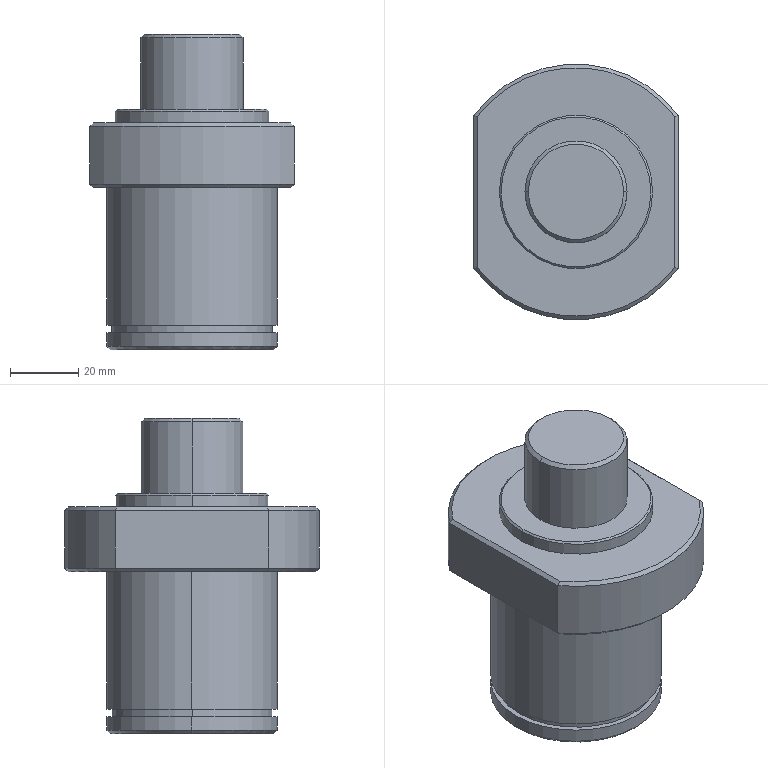Part | SolidWorks | features ICE 7, Chamfer 3, Extrusion 1 | 1 solid | 35 faces | box 60 x 75 x 92.5 mm | volume 189510 mm3 | plane 13 | cylinder 12 | cone 10 | commonest cylinder face diameters 50 x4 30 x2 45 x2 47 x2 75 x2
STEP:
#1=CARTESIAN_POINT('',(25.,0.,-79.5));
#2=VERTEX_POINT('',#1);
#3=CARTESIAN_POINT('',(-25.,0.,-79.5));
#4=VERTEX_POINT('',#3);
#5=CARTESIAN_POINT('',(0.,0.,-79.5));
#6=DIRECTION('',(0.,0.,1.));
#7=DIRECTION('',(-1.,0.,0.));
#8=AXIS2_PLACEMENT_3D('',#5,#6,#7);
#9=CIRCLE('',#8,25.);
#10=EDGE_CURVE('',#2,#4,#9,.T.);
#11=ORIENTED_EDGE('',*,*,#10,.T.);
#12=CARTESIAN_POINT('',(-25.,0.,-75.5));
#13=VERTEX_POINT('',#12);
#14=CARTESIAN_POINT('',(-25.,0.,-80.5));
#15=DIRECTION('',(0.,0.,1.));
#16=VECTOR('',#15,1000.);
#17=LINE('',#14,#16);
#18=EDGE_CURVE('',#4,#13,#17,.T.);
#19=ORIENTED_EDGE('',*,*,#18,.T.);
#20=CARTESIAN_POINT('',(25.,0.,-75.5));
#21=VERTEX_POINT('',#20);
#22=CARTESIAN_POINT('',(0.,0.,-75.5));
#23=DIRECTION('',(0.,0.,-1.));
#24=DIRECTION('',(-1.,0.,0.));
#25=AXIS2_PLACEMENT_3D('',#22,#23,#24);
#26=CIRCLE('',#25,25.);
#27=EDGE_CURVE('',#13,#21,#26,.T.);
#28=ORIENTED_EDGE('',*,*,#27,.T.);
#29=CARTESIAN_POINT('',(25.,0.,-80.5));
#30=DIRECTION('',(0.,0.,1.));
#31=VECTOR('',#30,1000.);
#32=LINE('',#29,#31);
#33=EDGE_CURVE('',#2,#21,#32,.T.);
#34=ORIENTED_EDGE('',*,*,#33,.F.);
#35=EDGE_LOOP('',(#11,#19,#28,#34));
#36=FACE_OUTER_BOUND('',#35,.T.);
#37=CARTESIAN_POINT('',(0.,0.,-80.5));
#38=DIRECTION('',(0.,0.,1.));
#39=DIRECTION('',(1.,0.,0.));
#40=AXIS2_PLACEMENT_3D('',#37,#38,#39);
#41=CYLINDRICAL_SURFACE('',#40,25.);
#42=ADVANCED_FACE('',(#36),#41,.T.);
#43=CARTESIAN_POINT('',(-24.,0.,-80.5));
#44=VERTEX_POINT('',#43);
#45=CARTESIAN_POINT('',(24.,0.,-80.5));
#46=VERTEX_POINT('',#45);
#47=CARTESIAN_POINT('',(0.,0.,-80.5));
#48=DIRECTION('',(0.,0.,-1.));
#49=DIRECTION('',(-1.,0.,0.));
#50=AXIS2_PLACEMENT_3D('',#47,#48,#49);
#51=CIRCLE('',#50,24.);
#52=EDGE_CURVE('',#44,#46,#51,.T.);
#53=ORIENTED_EDGE('',*,*,#52,.F.);
#54=CARTESIAN_POINT('',(-24.,0.,-80.5));
#55=DIRECTION('',(-0.7071,0.,0.7071));
#56=VECTOR('',#55,1000.);
#57=LINE('',#54,#56);
#58=EDGE_CURVE('',#44,#4,#57,.T.);
#59=ORIENTED_EDGE('',*,*,#58,.T.);
#60=ORIENTED_EDGE('',*,*,#10,.F.);
#61=CARTESIAN_POINT('',(24.,0.,-80.5));
#62=DIRECTION('',(0.7071,0.,0.7071));
#63=VECTOR('',#62,1000.);
#64=LINE('',#61,#63);
#65=EDGE_CURVE('',#46,#2,#64,.T.);
#66=ORIENTED_EDGE('',*,*,#65,.F.);
#67=EDGE_LOOP('',(#53,#59,#60,#66));
#68=FACE_OUTER_BOUND('',#67,.T.);
#69=CARTESIAN_POINT('',(0.,0.,-80.5));
#70=DIRECTION('',(0.,0.,1.));
#71=DIRECTION('',(1.,0.,0.));
#72=AXIS2_PLACEMENT_3D('',#69,#70,#71);
#73=CONICAL_SURFACE('',#72,24.,0.7854);
#74=ADVANCED_FACE('',(#68),#73,.T.);
#75=CARTESIAN_POINT('',(-23.5,0.,-73.3));
#76=VERTEX_POINT('',#75);
#77=CARTESIAN_POINT('',(23.5,0.,-73.3));
#78=VERTEX_POINT('',#77);
#79=CARTESIAN_POINT('',(0.,0.,-73.3));
#80=DIRECTION('',(0.,0.,-1.));
#81=DIRECTION('',(-1.,0.,0.));
#82=AXIS2_PLACEMENT_3D('',#79,#80,#81);
#83=CIRCLE('',#82,23.5);
#84=EDGE_CURVE('',#76,#78,#83,.T.);
#85=ORIENTED_EDGE('',*,*,#84,.T.);
#86=CARTESIAN_POINT('',(23.5,0.,-75.5));
#87=VERTEX_POINT('',#86);
#88=CARTESIAN_POINT('',(23.5,0.,-73.3));
#89=DIRECTION('',(0.,0.,-1.));
#90=VECTOR('',#89,1000.);
#91=LINE('',#88,#90);
#92=EDGE_CURVE('',#78,#87,#91,.T.);
#93=ORIENTED_EDGE('',*,*,#92,.T.);
#94=CARTESIAN_POINT('',(-23.5,0.,-75.5));
#95=VERTEX_POINT('',#94);
#96=CARTESIAN_POINT('',(0.,0.,-75.5));
#97=DIRECTION('',(0.,0.,-1.));
#98=DIRECTION('',(-1.,0.,0.));
#99=AXIS2_PLACEMENT_3D('',#96,#97,#98);
#100=CIRCLE('',#99,23.5);
#101=EDGE_CURVE('',#95,#87,#100,.T.);
#102=ORIENTED_EDGE('',*,*,#101,.F.);
#103=CARTESIAN_POINT('',(-23.5,0.,-73.3));
#104=DIRECTION('',(0.,0.,-1.));
#105=VECTOR('',#104,1000.);
#106=LINE('',#103,#105);
#107=EDGE_CURVE('',#76,#95,#106,.T.);
#108=ORIENTED_EDGE('',*,*,#107,.F.);
#109=EDGE_LOOP('',(#85,#93,#102,#108));
#110=FACE_OUTER_BOUND('',#109,.T.);
#111=CARTESIAN_POINT('',(0.,0.,-73.3));
#112=DIRECTION('',(0.,0.,-1.));
#113=DIRECTION('',(-1.,0.,0.));
#114=AXIS2_PLACEMENT_3D('',#111,#112,#113);
#115=CYLINDRICAL_SURFACE('',#114,23.5);
#116=ADVANCED_FACE('',(#110),#115,.T.);
#117=CARTESIAN_POINT('',(22.,0.,-10.));
#118=VERTEX_POINT('',#117);
#119=CARTESIAN_POINT('',(-22.,0.,-10.));
#120=VERTEX_POINT('',#119);
#121=CARTESIAN_POINT('',(0.,0.,-10.));
#122=DIRECTION('',(0.,0.,1.));
#123=DIRECTION('',(1.,0.,0.));
#124=AXIS2_PLACEMENT_3D('',#121,#122,#123);
#125=CIRCLE('',#124,22.);
#126=EDGE_CURVE('',#118,#120,#125,.T.);
#127=ORIENTED_EDGE('',*,*,#126,.F.);
#128=CARTESIAN_POINT('',(22.5,0.,-10.5));
#129=VERTEX_POINT('',#128);
#130=CARTESIAN_POINT('',(22.,0.,-10.));
#131=DIRECTION('',(0.7071,0.,-0.7071));
#132=VECTOR('',#131,1000.);
#133=LINE('',#130,#132);
#134=EDGE_CURVE('',#118,#129,#133,.T.);
#135=ORIENTED_EDGE('',*,*,#134,.T.);
#136=CARTESIAN_POINT('',(-22.5,0.,-10.5));
#137=VERTEX_POINT('',#136);
#138=CARTESIAN_POINT('',(0.,0.,-10.5));
#139=DIRECTION('',(0.,0.,-1.));
#140=DIRECTION('',(1.,0.,0.));
#141=AXIS2_PLACEMENT_3D('',#138,#139,#140);
#142=CIRCLE('',#141,22.5);
#143=EDGE_CURVE('',#137,#129,#142,.T.);
#144=ORIENTED_EDGE('',*,*,#143,.F.);
#145=CARTESIAN_POINT('',(-22.,0.,-10.));
#146=DIRECTION('',(-0.7071,0.,-0.7071));
#147=VECTOR('',#146,1000.);
#148=LINE('',#145,#147);
#149=EDGE_CURVE('',#120,#137,#148,.T.);
#150=ORIENTED_EDGE('',*,*,#149,.F.);
#151=EDGE_LOOP('',(#127,#135,#144,#150));
#152=FACE_OUTER_BOUND('',#151,.T.);
#153=CARTESIAN_POINT('',(0.,0.,-10.));
#154=DIRECTION('',(0.,0.,-1.));
#155=DIRECTION('',(-1.,0.,0.));
#156=AXIS2_PLACEMENT_3D('',#153,#154,#155);
#157=CONICAL_SURFACE('',#156,22.,0.7854);
#158=ADVANCED_FACE('',(#152),#157,.T.);
#159=CARTESIAN_POINT('',(14.,0.,12.));
#160=VERTEX_POINT('',#159);
#161=CARTESIAN_POINT('',(-14.,0.,12.));
#162=VERTEX_POINT('',#161);
#163=CARTESIAN_POINT('',(0.,0.,12.));
#164=DIRECTION('',(0.,0.,1.));
#165=DIRECTION('',(1.,0.,0.));
#166=AXIS2_PLACEMENT_3D('',#163,#164,#165);
#167=CIRCLE('',#166,14.);
#168=EDGE_CURVE('',#160,#162,#167,.T.);
#169=ORIENTED_EDGE('',*,*,#168,.F.);
#170=CARTESIAN_POINT('',(15.,0.,11.));
#171=VERTEX_POINT('',#170);
#172=CARTESIAN_POINT('',(14.,0.,12.));
#173=DIRECTION('',(0.7071,0.,-0.7071));
#174=VECTOR('',#173,1000.);
#175=LINE('',#172,#174);
#176=EDGE_CURVE('',#160,#171,#175,.T.);
#177=ORIENTED_EDGE('',*,*,#176,.T.);
#178=CARTESIAN_POINT('',(-15.,0.,11.));
#179=VERTEX_POINT('',#178);
#180=CARTESIAN_POINT('',(0.,0.,11.));
#181=DIRECTION('',(0.,0.,-1.));
#182=DIRECTION('',(1.,0.,0.));
#183=AXIS2_PLACEMENT_3D('',#180,#181,#182);
#184=CIRCLE('',#183,15.);
#185=EDGE_CURVE('',#179,#171,#184,.T.);
#186=ORIENTED_EDGE('',*,*,#185,.F.);
#187=CARTESIAN_POINT('',(-14.,0.,12.));
#188=DIRECTION('',(-0.7071,0.,-0.7071));
#189=VECTOR('',#188,1000.);
#190=LINE('',#187,#189);
#191=EDGE_CURVE('',#162,#179,#190,.T.);
#192=ORIENTED_EDGE('',*,*,#191,.F.);
#193=EDGE_LOOP('',(#169,#177,#186,#192));
#194=FACE_OUTER_BOUND('',#193,.T.);
#195=CARTESIAN_POINT('',(0.,0.,12.));
#196=DIRECTION('',(0.,0.,-1.));
#197=DIRECTION('',(-1.,0.,0.));
#198=AXIS2_PLACEMENT_3D('',#195,#196,#197);
#199=CONICAL_SURFACE('',#198,14.,0.7854);
#200=ADVANCED_FACE('',(#194),#199,.T.);
#201=ORIENTED_EDGE('',*,*,#185,.T.);
#202=CARTESIAN_POINT('',(15.,0.,-10.));
#203=VERTEX_POINT('',#202);
#204=CARTESIAN_POINT('',(15.,0.,12.));
#205=DIRECTION('',(0.,0.,-1.));
#206=VECTOR('',#205,1000.);
#207=LINE('',#204,#206);
#208=EDGE_CURVE('',#171,#203,#207,.T.);
#209=ORIENTED_EDGE('',*,*,#208,.T.);
#210=CARTESIAN_POINT('',(-15.,0.,-10.));
#211=VERTEX_POINT('',#210);
#212=CARTESIAN_POINT('',(0.,0.,-10.));
#213=DIRECTION('',(0.,0.,1.));
#214=DIRECTION('',(1.,0.,0.));
#215=AXIS2_PLACEMENT_3D('',#212,#213,#214);
#216=CIRCLE('',#215,15.);
#217=EDGE_CURVE('',#203,#211,#216,.T.);
#218=ORIENTED_EDGE('',*,*,#217,.T.);
#219=CARTESIAN_POINT('',(-15.,0.,12.));
#220=DIRECTION('',(0.,0.,-1.));
#221=VECTOR('',#220,1000.);
#222=LINE('',#219,#221);
#223=EDGE_CURVE('',#179,#211,#222,.T.);
#224=ORIENTED_EDGE('',*,*,#223,.F.);
#225=EDGE_LOOP('',(#201,#209,#218,#224));
#226=FACE_OUTER_BOUND('',#225,.T.);
#227=CARTESIAN_POINT('',(0.,0.,12.));
#228=DIRECTION('',(0.,0.,-1.));
#229=DIRECTION('',(-1.,0.,0.));
#230=AXIS2_PLACEMENT_3D('',#227,#228,#229);
#231=CYLINDRICAL_SURFACE('',#230,15.);
#232=ADVANCED_FACE('',(#226),#231,.T.);
#233=ORIENTED_EDGE('',*,*,#143,.T.);
#234=CARTESIAN_POINT('',(22.5,0.,-14.));
#235=VERTEX_POINT('',#234);
#236=CARTESIAN_POINT('',(22.5,0.,-10.));
#237=DIRECTION('',(0.,0.,-1.));
#238=VECTOR('',#237,1000.);
#239=LINE('',#236,#238);
#240=EDGE_CURVE('',#129,#235,#239,.T.);
#241=ORIENTED_EDGE('',*,*,#240,.T.);
#242=CARTESIAN_POINT('',(-22.5,0.,-14.));
#243=VERTEX_POINT('',#242);
#244=CARTESIAN_POINT('',(0.,0.,-14.));
#245=DIRECTION('',(0.,0.,1.));
#246=DIRECTION('',(1.,0.,0.));
#247=AXIS2_PLACEMENT_3D('',#244,#245,#246);
#248=CIRCLE('',#247,22.5);
#249=EDGE_CURVE('',#235,#243,#248,.T.);
#250=ORIENTED_EDGE('',*,*,#249,.T.);
#251=CARTESIAN_POINT('',(-22.5,0.,-10.));
#252=DIRECTION('',(0.,0.,-1.));
#253=VECTOR('',#252,1000.);
#254=LINE('',#251,#253);
#255=EDGE_CURVE('',#137,#243,#254,.T.);
#256=ORIENTED_EDGE('',*,*,#255,.F.);
#257=EDGE_LOOP('',(#233,#241,#250,#256));
#258=FACE_OUTER_BOUND('',#257,.T.);
#259=CARTESIAN_POINT('',(0.,0.,-10.));
#260=DIRECTION('',(0.,0.,-1.));
#261=DIRECTION('',(-1.,0.,0.));
#262=AXIS2_PLACEMENT_3D('',#259,#260,#261);
#263=CYLINDRICAL_SURFACE('',#262,22.5);
#264=ADVANCED_FACE('',(#258),#263,.T.);
#265=CARTESIAN_POINT('',(-25.,0.,-73.3));
#266=VERTEX_POINT('',#265);
#267=CARTESIAN_POINT('',(25.,0.,-73.3));
#268=VERTEX_POINT('',#267);
#269=CARTESIAN_POINT('',(0.,0.,-73.3));
#270=DIRECTION('',(0.,0.,-1.));
#271=DIRECTION('',(-1.,0.,0.));
#272=AXIS2_PLACEMENT_3D('',#269,#270,#271);
#273=CIRCLE('',#272,25.);
#274=EDGE_CURVE('',#266,#268,#273,.T.);
#275=ORIENTED_EDGE('',*,*,#274,.F.);
#276=CARTESIAN_POINT('',(-25.,0.,-33.));
#277=VERTEX_POINT('',#276);
#278=CARTESIAN_POINT('',(-25.,0.,-80.5));
#279=DIRECTION('',(0.,0.,1.));
#280=VECTOR('',#279,1000.);
#281=LINE('',#278,#280);
#282=EDGE_CURVE('',#266,#277,#281,.T.);
#283=ORIENTED_EDGE('',*,*,#282,.T.);
#284=CARTESIAN_POINT('',(25.,0.,-33.));
#285=VERTEX_POINT('',#284);
#286=CARTESIAN_POINT('',(0.,0.,-33.));
#287=DIRECTION('',(0.,0.,1.));
#288=DIRECTION('',(1.,0.,0.));
#289=AXIS2_PLACEMENT_3D('',#286,#287,#288);
#290=CIRCLE('',#289,25.);
#291=EDGE_CURVE('',#285,#277,#290,.T.);
#292=ORIENTED_EDGE('',*,*,#291,.F.);
#293=CARTESIAN_POINT('',(25.,0.,-80.5));
#294=DIRECTION('',(0.,0.,1.));
#295=VECTOR('',#294,1000.);
#296=LINE('',#293,#295);
#297=EDGE_CURVE('',#268,#285,#296,.T.);
#298=ORIENTED_EDGE('',*,*,#297,.F.);
#299=EDGE_LOOP('',(#275,#283,#292,#298));
#300=FACE_OUTER_BOUND('',#299,.T.);
#301=CARTESIAN_POINT('',(0.,0.,-80.5));
#302=DIRECTION('',(0.,0.,1.));
#303=DIRECTION('',(1.,0.,0.));
#304=AXIS2_PLACEMENT_3D('',#301,#302,#303);
#305=CYLINDRICAL_SURFACE('',#304,25.);
#306=ADVANCED_FACE('',(#300),#305,.T.);
#307=ORIENTED_EDGE('',*,*,#282,.F.);
#308=CARTESIAN_POINT('',(0.,0.,-73.3));
#309=DIRECTION('',(0.,0.,-1.));
#310=DIRECTION('',(-1.,0.,0.));
#311=AXIS2_PLACEMENT_3D('',#308,#309,#310);
#312=CIRCLE('',#311,25.);
#313=EDGE_CURVE('',#268,#266,#312,.T.);
#314=ORIENTED_EDGE('',*,*,#313,.F.);
#315=ORIENTED_EDGE('',*,*,#297,.T.);
#316=CARTESIAN_POINT('',(0.,0.,-33.));
#317=DIRECTION('',(0.,0.,1.));
#318=DIRECTION('',(1.,0.,0.));
#319=AXIS2_PLACEMENT_3D('',#316,#317,#318);
#320=CIRCLE('',#319,25.);
#321=EDGE_CURVE('',#277,#285,#320,.T.);
#322=ORIENTED_EDGE('',*,*,#321,.F.);
#323=EDGE_LOOP('',(#307,#314,#315,#322));
#324=FACE_OUTER_BOUND('',#323,.T.);
#325=CARTESIAN_POINT('',(0.,0.,-80.5));
#326=DIRECTION('',(0.,0.,1.));
#327=DIRECTION('',(1.,0.,0.));
#328=AXIS2_PLACEMENT_3D('',#325,#326,#327);
#329=CYLINDRICAL_SURFACE('',#328,25.);
#330=ADVANCED_FACE('',(#324),#329,.T.);
#331=ORIENTED_EDGE('',*,*,#240,.F.);
#332=CARTESIAN_POINT('',(0.,0.,-10.5));
#333=DIRECTION('',(0.,0.,-1.));
#334=DIRECTION('',(1.,0.,0.));
#335=AXIS2_PLACEMENT_3D('',#332,#333,#334);
#336=CIRCLE('',#335,22.5);
#337=EDGE_CURVE('',#129,#137,#336,.T.);
#338=ORIENTED_EDGE('',*,*,#337,.T.);
#339=ORIENTED_EDGE('',*,*,#255,.T.);
#340=CARTESIAN_POINT('',(0.,0.,-14.));
#341=DIRECTION('',(0.,0.,1.));
#342=DIRECTION('',(1.,0.,0.));
#343=AXIS2_PLACEMENT_3D('',#340,#341,#342);
#344=CIRCLE('',#343,22.5);
#345=EDGE_CURVE('',#243,#235,#344,.T.);
#346=ORIENTED_EDGE('',*,*,#345,.T.);
#347=EDGE_LOOP('',(#331,#338,#339,#346));
#348=FACE_OUTER_BOUND('',#347,.T.);
#349=CARTESIAN_POINT('',(0.,0.,-10.));
#350=DIRECTION('',(0.,0.,-1.));
#351=DIRECTION('',(-1.,0.,0.));
#352=AXIS2_PLACEMENT_3D('',#349,#350,#351);
#353=CYLINDRICAL_SURFACE('',#352,22.5);
#354=ADVANCED_FACE('',(#348),#353,.T.);
#355=CARTESIAN_POINT('',(0.,0.,-10.));
#356=DIRECTION('',(0.,0.,1.));
#357=DIRECTION('',(1.,0.,0.));
#358=AXIS2_PLACEMENT_3D('',#355,#356,#357);
#359=CIRCLE('',#358,22.);
#360=EDGE_CURVE('',#120,#118,#359,.T.);
#361=ORIENTED_EDGE('',*,*,#360,.T.);
#362=ORIENTED_EDGE('',*,*,#126,.T.);
#363=EDGE_LOOP('',(#361,#362));
#364=FACE_OUTER_BOUND('',#363,.T.);
#365=CARTESIAN_POINT('',(0.,0.,-10.));
#366=DIRECTION('',(0.,0.,1.));
#367=DIRECTION('',(1.,0.,0.));
#368=AXIS2_PLACEMENT_3D('',#365,#366,#367);
#369=CIRCLE('',#368,15.);
#370=EDGE_CURVE('',#211,#203,#369,.T.);
#371=ORIENTED_EDGE('',*,*,#370,.F.);
#372=ORIENTED_EDGE('',*,*,#217,.F.);
#373=EDGE_LOOP('',(#371,#372));
#374=FACE_BOUND('',#373,.T.);
#375=CARTESIAN_POINT('',(0.,0.,-10.));
#376=DIRECTION('',(0.,0.,1.));
#377=DIRECTION('',(1.,0.,0.));
#378=AXIS2_PLACEMENT_3D('',#375,#376,#377);
#379=PLANE('',#378);
#380=ADVANCED_FACE('',(#364,#374),#379,.T.);
#381=CARTESIAN_POINT('',(0.,0.,12.));
#382=DIRECTION('',(0.,0.,1.));
#383=DIRECTION('',(1.,0.,0.));
#384=AXIS2_PLACEMENT_3D('',#381,#382,#383);
#385=CIRCLE('',#384,14.);
#386=EDGE_CURVE('',#162,#160,#385,.T.);
#387=ORIENTED_EDGE('',*,*,#386,.T.);
#388=ORIENTED_EDGE('',*,*,#168,.T.);
#389=EDGE_LOOP('',(#387,#388));
#390=FACE_OUTER_BOUND('',#389,.T.);
#391=CARTESIAN_POINT('',(0.,0.,12.));
#392=DIRECTION('',(0.,0.,1.));
#393=DIRECTION('',(1.,0.,0.));
#394=AXIS2_PLACEMENT_3D('',#391,#392,#393);
#395=PLANE('',#394);
#396=ADVANCED_FACE('',(#390),#395,.T.);
#397=ORIENTED_EDGE('',*,*,#208,.F.);
#398=CARTESIAN_POINT('',(0.,0.,11.));
#399=DIRECTION('',(0.,0.,-1.));
#400=DIRECTION('',(1.,0.,0.));
#401=AXIS2_PLACEMENT_3D('',#398,#399,#400);
#402=CIRCLE('',#401,15.);
#403=EDGE_CURVE('',#171,#179,#402,.T.);
#404=ORIENTED_EDGE('',*,*,#403,.T.);
#405=ORIENTED_EDGE('',*,*,#223,.T.);
#406=ORIENTED_EDGE('',*,*,#370,.T.);
#407=EDGE_LOOP('',(#397,#404,#405,#406));
#408=FACE_OUTER_BOUND('',#407,.T.);
#409=CARTESIAN_POINT('',(0.,0.,12.));
#410=DIRECTION('',(0.,0.,-1.));
#411=DIRECTION('',(-1.,0.,0.));
#412=AXIS2_PLACEMENT_3D('',#409,#410,#411);
#413=CYLINDRICAL_SURFACE('',#412,15.);
#414=ADVANCED_FACE('',(#408),#413,.T.);
#415=ORIENTED_EDGE('',*,*,#176,.F.);
#416=ORIENTED_EDGE('',*,*,#386,.F.);
#417=ORIENTED_EDGE('',*,*,#191,.T.);
#418=ORIENTED_EDGE('',*,*,#403,.F.);
#419=EDGE_LOOP('',(#415,#416,#417,#418));
#420=FACE_OUTER_BOUND('',#419,.T.);
#421=CARTESIAN_POINT('',(0.,0.,12.));
#422=DIRECTION('',(0.,0.,-1.));
#423=DIRECTION('',(-1.,0.,0.));
#424=AXIS2_PLACEMENT_3D('',#421,#422,#423);
#425=CONICAL_SURFACE('',#424,14.,0.7854);
#426=ADVANCED_FACE('',(#420),#425,.T.);
#427=ORIENTED_EDGE('',*,*,#134,.F.);
#428=ORIENTED_EDGE('',*,*,#360,.F.);
#429=ORIENTED_EDGE('',*,*,#149,.T.);
#430=ORIENTED_EDGE('',*,*,#337,.F.);
#431=EDGE_LOOP('',(#427,#428,#429,#430));
#432=FACE_OUTER_BOUND('',#431,.T.);
#433=CARTESIAN_POINT('',(0.,0.,-10.));
#434=DIRECTION('',(0.,0.,-1.));
#435=DIRECTION('',(-1.,0.,0.));
#436=AXIS2_PLACEMENT_3D('',#433,#434,#435);
#437=CONICAL_SURFACE('',#436,22.,0.7854);
#438=ADVANCED_FACE('',(#432),#437,.T.);
#439=CARTESIAN_POINT('',(-29.,22.164,-14.));
#440=VERTEX_POINT('',#439);
#441=CARTESIAN_POINT('',(-29.,-22.164,-14.));
#442=VERTEX_POINT('',#441);
#443=CARTESIAN_POINT('',(-29.,0.,-14.));
#444=DIRECTION('',(0.,-1.,0.));
#445=VECTOR('',#444,1000.);
#446=LINE('',#443,#445);
#447=EDGE_CURVE('',#440,#442,#446,.T.);
#448=ORIENTED_EDGE('',*,*,#447,.T.);
#449=CARTESIAN_POINT('',(29.,-22.164,-14.));
#450=VERTEX_POINT('',#449);
#451=CARTESIAN_POINT('',(0.,0.,-14.));
#452=DIRECTION('',(0.,0.,1.));
#453=DIRECTION('',(1.,0.,0.));
#454=AXIS2_PLACEMENT_3D('',#451,#452,#453);
#455=CIRCLE('',#454,36.5);
#456=EDGE_CURVE('',#442,#450,#455,.T.);
#457=ORIENTED_EDGE('',*,*,#456,.T.);
#458=CARTESIAN_POINT('',(29.,22.164,-14.));
#459=VERTEX_POINT('',#458);
#460=CARTESIAN_POINT('',(29.,0.,-14.));
#461=DIRECTION('',(0.,1.,0.));
#462=VECTOR('',#461,1000.);
#463=LINE('',#460,#462);
#464=EDGE_CURVE('',#450,#459,#463,.T.);
#465=ORIENTED_EDGE('',*,*,#464,.T.);
#466=CARTESIAN_POINT('',(0.,0.,-14.));
#467=DIRECTION('',(0.,0.,1.));
#468=DIRECTION('',(1.,0.,0.));
#469=AXIS2_PLACEMENT_3D('',#466,#467,#468);
#470=CIRCLE('',#469,36.5);
#471=EDGE_CURVE('',#459,#440,#470,.T.);
#472=ORIENTED_EDGE('',*,*,#471,.T.);
#473=EDGE_LOOP('',(#448,#457,#465,#472));
#474=FACE_OUTER_BOUND('',#473,.T.);
#475=ORIENTED_EDGE('',*,*,#345,.F.);
#476=ORIENTED_EDGE('',*,*,#249,.F.);
#477=EDGE_LOOP('',(#475,#476));
#478=FACE_BOUND('',#477,.T.);
#479=CARTESIAN_POINT('',(0.,0.,-14.));
#480=DIRECTION('',(0.,0.,1.));
#481=DIRECTION('',(1.,0.,0.));
#482=AXIS2_PLACEMENT_3D('',#479,#480,#481);
#483=PLANE('',#482);
#484=ADVANCED_FACE('',(#474,#478),#483,.T.);
#485=CARTESIAN_POINT('',(-29.,-22.164,-33.));
#486=VERTEX_POINT('',#485);
#487=CARTESIAN_POINT('',(-29.,22.164,-33.));
#488=VERTEX_POINT('',#487);
#489=CARTESIAN_POINT('',(-29.,22.5,-33.));
#490=DIRECTION('',(0.,1.,0.));
#491=VECTOR('',#490,1000.);
#492=LINE('',#489,#491);
#493=EDGE_CURVE('',#486,#488,#492,.T.);
#494=ORIENTED_EDGE('',*,*,#493,.T.);
#495=CARTESIAN_POINT('',(29.,22.164,-33.));
#496=VERTEX_POINT('',#495);
#497=CARTESIAN_POINT('',(0.,0.,-33.));
#498=DIRECTION('',(0.,0.,-1.));
#499=DIRECTION('',(1.,0.,0.));
#500=AXIS2_PLACEMENT_3D('',#497,#498,#499);
#501=CIRCLE('',#500,36.5);
#502=EDGE_CURVE('',#488,#496,#501,.T.);
#503=ORIENTED_EDGE('',*,*,#502,.T.);
#504=CARTESIAN_POINT('',(29.,-22.164,-33.));
#505=VERTEX_POINT('',#504);
#506=CARTESIAN_POINT('',(29.,-22.5,-33.));
#507=DIRECTION('',(0.,-1.,0.));
#508=VECTOR('',#507,1000.);
#509=LINE('',#506,#508);
#510=EDGE_CURVE('',#496,#505,#509,.T.);
#511=ORIENTED_EDGE('',*,*,#510,.T.);
#512=CARTESIAN_POINT('',(0.,0.,-33.));
#513=DIRECTION('',(0.,0.,-1.));
#514=DIRECTION('',(1.,0.,0.));
#515=AXIS2_PLACEMENT_3D('',#512,#513,#514);
#516=CIRCLE('',#515,36.5);
#517=EDGE_CURVE('',#505,#486,#516,.T.);
#518=ORIENTED_EDGE('',*,*,#517,.T.);
#519=EDGE_LOOP('',(#494,#503,#511,#518));
#520=FACE_OUTER_BOUND('',#519,.T.);
#521=ORIENTED_EDGE('',*,*,#291,.T.);
#522=ORIENTED_EDGE('',*,*,#321,.T.);
#523=EDGE_LOOP('',(#521,#522));
#524=FACE_BOUND('',#523,.T.);
#525=CARTESIAN_POINT('',(0.,0.,-33.));
#526=DIRECTION('',(0.,0.,1.));
#527=DIRECTION('',(1.,0.,0.));
#528=AXIS2_PLACEMENT_3D('',#525,#526,#527);
#529=PLANE('',#528);
#530=ADVANCED_FACE('',(#520,#524),#529,.F.);
#531=CARTESIAN_POINT('',(30.,22.5,-32.));
#532=VERTEX_POINT('',#531);
#533=CARTESIAN_POINT('',(30.,22.5,-32.));
#534=CARTESIAN_POINT('',(29.667,22.389,-32.333));
#535=CARTESIAN_POINT('',(29.333,22.277,-32.667));
#536=CARTESIAN_POINT('',(29.,22.164,-33.));
#537=B_SPLINE_CURVE_WITH_KNOTS('',3,(#533,#534,#535,#536),.UNSPECIFIED.,.F.,.F.,(4,4),(0.,0.001454),.UNSPECIFIED.);
#538=EDGE_CURVE('',#532,#496,#537,.T.);
#539=ORIENTED_EDGE('',*,*,#538,.T.);
#540=ORIENTED_EDGE('',*,*,#502,.F.);
#541=CARTESIAN_POINT('',(-30.,22.5,-32.));
#542=VERTEX_POINT('',#541);
#543=CARTESIAN_POINT('',(-29.,22.164,-33.));
#544=CARTESIAN_POINT('',(-29.333,22.277,-32.667));
#545=CARTESIAN_POINT('',(-29.667,22.389,-32.333));
#546=CARTESIAN_POINT('',(-30.,22.5,-32.));
#547=B_SPLINE_CURVE_WITH_KNOTS('',3,(#543,#544,#545,#546),.UNSPECIFIED.,.F.,.F.,(4,4),(0.,0.001454),.UNSPECIFIED.);
#548=EDGE_CURVE('',#488,#542,#547,.T.);
#549=ORIENTED_EDGE('',*,*,#548,.T.);
#550=CARTESIAN_POINT('',(0.,0.,-32.));
#551=DIRECTION('',(0.,0.,1.));
#552=DIRECTION('',(1.,0.,0.));
#553=AXIS2_PLACEMENT_3D('',#550,#551,#552);
#554=CIRCLE('',#553,37.5);
#555=EDGE_CURVE('',#532,#542,#554,.T.);
#556=ORIENTED_EDGE('',*,*,#555,.F.);
#557=EDGE_LOOP('',(#539,#540,#549,#556));
#558=FACE_OUTER_BOUND('',#557,.T.);
#559=CARTESIAN_POINT('',(0.,0.,-32.));
#560=DIRECTION('',(0.,0.,1.));
#561=DIRECTION('',(1.,0.,0.));
#562=AXIS2_PLACEMENT_3D('',#559,#560,#561);
#563=CONICAL_SURFACE('',#562,37.5,0.7854);
#564=ADVANCED_FACE('',(#558),#563,.T.);
#565=CARTESIAN_POINT('',(-30.,-22.5,-32.));
#566=VERTEX_POINT('',#565);
#567=CARTESIAN_POINT('',(-29.,-22.164,-33.));
#568=CARTESIAN_POINT('',(-29.333,-22.277,-32.667));
#569=CARTESIAN_POINT('',(-29.667,-22.389,-32.333));
#570=CARTESIAN_POINT('',(-30.,-22.5,-32.));
#571=B_SPLINE_CURVE_WITH_KNOTS('',3,(#567,#568,#569,#570),.UNSPECIFIED.,.F.,.F.,(4,4),(0.,0.001454),.UNSPECIFIED.);
#572=EDGE_CURVE('',#486,#566,#571,.T.);
#573=ORIENTED_EDGE('',*,*,#572,.F.);
#574=ORIENTED_EDGE('',*,*,#517,.F.);
#575=CARTESIAN_POINT('',(30.,-22.5,-32.));
#576=VERTEX_POINT('',#575);
#577=CARTESIAN_POINT('',(30.,-22.5,-32.));
#578=CARTESIAN_POINT('',(29.667,-22.389,-32.333));
#579=CARTESIAN_POINT('',(29.333,-22.277,-32.667));
#580=CARTESIAN_POINT('',(29.,-22.164,-33.));
#581=B_SPLINE_CURVE_WITH_KNOTS('',3,(#577,#578,#579,#580),.UNSPECIFIED.,.F.,.F.,(4,4),(0.,0.001454),.UNSPECIFIED.);
#582=EDGE_CURVE('',#576,#505,#581,.T.);
#583=ORIENTED_EDGE('',*,*,#582,.F.);
#584=CARTESIAN_POINT('',(0.,0.,-32.));
#585=DIRECTION('',(0.,0.,1.));
#586=DIRECTION('',(1.,0.,0.));
#587=AXIS2_PLACEMENT_3D('',#584,#585,#586);
#588=CIRCLE('',#587,37.5);
#589=EDGE_CURVE('',#566,#576,#588,.T.);
#590=ORIENTED_EDGE('',*,*,#589,.F.);
#591=EDGE_LOOP('',(#573,#574,#583,#590));
#592=FACE_OUTER_BOUND('',#591,.T.);
#593=CARTESIAN_POINT('',(0.,0.,-32.));
#594=DIRECTION('',(0.,0.,1.));
#595=DIRECTION('',(1.,0.,0.));
#596=AXIS2_PLACEMENT_3D('',#593,#594,#595);
#597=CONICAL_SURFACE('',#596,37.5,0.7854);
#598=ADVANCED_FACE('',(#592),#597,.T.);
#599=ORIENTED_EDGE('',*,*,#572,.T.);
#600=CARTESIAN_POINT('',(-30.,-22.5,-32.));
#601=DIRECTION('',(0.,-1.,0.));
#602=VECTOR('',#601,1000.);
#603=LINE('',#600,#602);
#604=EDGE_CURVE('',#542,#566,#603,.T.);
#605=ORIENTED_EDGE('',*,*,#604,.F.);
#606=ORIENTED_EDGE('',*,*,#548,.F.);
#607=ORIENTED_EDGE('',*,*,#493,.F.);
#608=EDGE_LOOP('',(#599,#605,#606,#607));
#609=FACE_OUTER_BOUND('',#608,.T.);
#610=CARTESIAN_POINT('',(-30.,-45.659,-32.));
#611=DIRECTION('',(-0.7071,0.,-0.7071));
#612=DIRECTION('',(0.,1.,0.));
#613=AXIS2_PLACEMENT_3D('',#610,#611,#612);
#614=PLANE('',#613);
#615=ADVANCED_FACE('',(#609),#614,.T.);
#616=ORIENTED_EDGE('',*,*,#582,.T.);
#617=ORIENTED_EDGE('',*,*,#510,.F.);
#618=ORIENTED_EDGE('',*,*,#538,.F.);
#619=CARTESIAN_POINT('',(30.,22.5,-32.));
#620=DIRECTION('',(0.,1.,0.));
#621=VECTOR('',#620,1000.);
#622=LINE('',#619,#621);
#623=EDGE_CURVE('',#576,#532,#622,.T.);
#624=ORIENTED_EDGE('',*,*,#623,.F.);
#625=EDGE_LOOP('',(#616,#617,#618,#624));
#626=FACE_OUTER_BOUND('',#625,.T.);
#627=CARTESIAN_POINT('',(30.,-45.659,-32.));
#628=DIRECTION('',(0.7071,0.,-0.7071));
#629=DIRECTION('',(0.,-1.,0.));
#630=AXIS2_PLACEMENT_3D('',#627,#628,#629);
#631=PLANE('',#630);
#632=ADVANCED_FACE('',(#626),#631,.T.);
#633=CARTESIAN_POINT('',(-30.,-22.5,-15.));
#634=VERTEX_POINT('',#633);
#635=CARTESIAN_POINT('',(-30.,-22.5,-33.));
#636=DIRECTION('',(0.,0.,-1.));
#637=VECTOR('',#636,1000.);
#638=LINE('',#635,#637);
#639=EDGE_CURVE('',#634,#566,#638,.T.);
#640=ORIENTED_EDGE('',*,*,#639,.F.);
#641=CARTESIAN_POINT('',(-30.,22.5,-15.));
#642=VERTEX_POINT('',#641);
#643=CARTESIAN_POINT('',(-30.,-45.659,-15.));
#644=DIRECTION('',(0.,1.,0.));
#645=VECTOR('',#644,1000.);
#646=LINE('',#643,#645);
#647=EDGE_CURVE('',#634,#642,#646,.T.);
#648=ORIENTED_EDGE('',*,*,#647,.T.);
#649=CARTESIAN_POINT('',(-30.,22.5,-33.));
#650=DIRECTION('',(0.,0.,1.));
#651=VECTOR('',#650,1000.);
#652=LINE('',#649,#651);
#653=EDGE_CURVE('',#542,#642,#652,.T.);
#654=ORIENTED_EDGE('',*,*,#653,.F.);
#655=ORIENTED_EDGE('',*,*,#604,.T.);
#656=EDGE_LOOP('',(#640,#648,#654,#655));
#657=FACE_OUTER_BOUND('',#656,.T.);
#658=CARTESIAN_POINT('',(-30.,-45.659,-7.5));
#659=DIRECTION('',(-1.,0.,0.));
#660=DIRECTION('',(0.,0.,1.));
#661=AXIS2_PLACEMENT_3D('',#658,#659,#660);
#662=PLANE('',#661);
#663=ADVANCED_FACE('',(#657),#662,.T.);
#664=CARTESIAN_POINT('',(30.,22.5,-15.));
#665=VERTEX_POINT('',#664);
#666=CARTESIAN_POINT('',(30.,22.5,-33.));
#667=DIRECTION('',(0.,0.,-1.));
#668=VECTOR('',#667,1000.);
#669=LINE('',#666,#668);
#670=EDGE_CURVE('',#665,#532,#669,.T.);
#671=ORIENTED_EDGE('',*,*,#670,.F.);
#672=CARTESIAN_POINT('',(30.,-22.5,-15.));
#673=VERTEX_POINT('',#672);
#674=CARTESIAN_POINT('',(30.,-45.659,-15.));
#675=DIRECTION('',(0.,-1.,0.));
#676=VECTOR('',#675,1000.);
#677=LINE('',#674,#676);
#678=EDGE_CURVE('',#665,#673,#677,.T.);
#679=ORIENTED_EDGE('',*,*,#678,.T.);
#680=CARTESIAN_POINT('',(30.,-22.5,-33.));
#681=DIRECTION('',(0.,0.,1.));
#682=VECTOR('',#681,1000.);
#683=LINE('',#680,#682);
#684=EDGE_CURVE('',#576,#673,#683,.T.);
#685=ORIENTED_EDGE('',*,*,#684,.F.);
#686=ORIENTED_EDGE('',*,*,#623,.T.);
#687=EDGE_LOOP('',(#671,#679,#685,#686));
#688=FACE_OUTER_BOUND('',#687,.T.);
#689=CARTESIAN_POINT('',(30.,-45.659,-7.5));
#690=DIRECTION('',(1.,0.,0.));
#691=DIRECTION('',(0.,0.,-1.));
#692=AXIS2_PLACEMENT_3D('',#689,#690,#691);
#693=PLANE('',#692);
#694=ADVANCED_FACE('',(#688),#693,.T.);
#695=ORIENTED_EDGE('',*,*,#684,.T.);
#696=CARTESIAN_POINT('',(0.,0.,-15.));
#697=DIRECTION('',(0.,0.,-1.));
#698=DIRECTION('',(1.,0.,0.));
#699=AXIS2_PLACEMENT_3D('',#696,#697,#698);
#700=CIRCLE('',#699,37.5);
#701=EDGE_CURVE('',#673,#634,#700,.T.);
#702=ORIENTED_EDGE('',*,*,#701,.T.);
#703=ORIENTED_EDGE('',*,*,#639,.T.);
#704=ORIENTED_EDGE('',*,*,#589,.T.);
#705=EDGE_LOOP('',(#695,#702,#703,#704));
#706=FACE_OUTER_BOUND('',#705,.T.);
#707=CARTESIAN_POINT('',(0.,0.,-33.));
#708=DIRECTION('',(0.,0.,1.));
#709=DIRECTION('',(1.,0.,0.));
#710=AXIS2_PLACEMENT_3D('',#707,#708,#709);
#711=CYLINDRICAL_SURFACE('',#710,37.5);
#712=ADVANCED_FACE('',(#706),#711,.T.);
#713=ORIENTED_EDGE('',*,*,#653,.T.);
#714=CARTESIAN_POINT('',(0.,0.,-15.));
#715=DIRECTION('',(0.,0.,-1.));
#716=DIRECTION('',(1.,0.,0.));
#717=AXIS2_PLACEMENT_3D('',#714,#715,#716);
#718=CIRCLE('',#717,37.5);
#719=EDGE_CURVE('',#642,#665,#718,.T.);
#720=ORIENTED_EDGE('',*,*,#719,.T.);
#721=ORIENTED_EDGE('',*,*,#670,.T.);
#722=ORIENTED_EDGE('',*,*,#555,.T.);
#723=EDGE_LOOP('',(#713,#720,#721,#722));
#724=FACE_OUTER_BOUND('',#723,.T.);
#725=CARTESIAN_POINT('',(0.,0.,-33.));
#726=DIRECTION('',(0.,0.,1.));
#727=DIRECTION('',(1.,0.,0.));
#728=AXIS2_PLACEMENT_3D('',#725,#726,#727);
#729=CYLINDRICAL_SURFACE('',#728,37.5);
#730=ADVANCED_FACE('',(#724),#729,.T.);
#731=CARTESIAN_POINT('',(30.,22.5,-15.));
#732=CARTESIAN_POINT('',(29.667,22.389,-14.667));
#733=CARTESIAN_POINT('',(29.333,22.277,-14.333));
#734=CARTESIAN_POINT('',(29.,22.164,-14.));
#735=B_SPLINE_CURVE_WITH_KNOTS('',3,(#731,#732,#733,#734),.UNSPECIFIED.,.F.,.F.,(4,4),(0.,0.001454),.UNSPECIFIED.);
#736=EDGE_CURVE('',#665,#459,#735,.T.);
#737=ORIENTED_EDGE('',*,*,#736,.F.);
#738=ORIENTED_EDGE('',*,*,#719,.F.);
#739=CARTESIAN_POINT('',(-29.,22.164,-14.));
#740=CARTESIAN_POINT('',(-29.333,22.277,-14.333));
#741=CARTESIAN_POINT('',(-29.667,22.389,-14.667));
#742=CARTESIAN_POINT('',(-30.,22.5,-15.));
#743=B_SPLINE_CURVE_WITH_KNOTS('',3,(#739,#740,#741,#742),.UNSPECIFIED.,.F.,.F.,(4,4),(0.,0.001454),.UNSPECIFIED.);
#744=EDGE_CURVE('',#440,#642,#743,.T.);
#745=ORIENTED_EDGE('',*,*,#744,.F.);
#746=ORIENTED_EDGE('',*,*,#471,.F.);
#747=EDGE_LOOP('',(#737,#738,#745,#746));
#748=FACE_OUTER_BOUND('',#747,.T.);
#749=CARTESIAN_POINT('',(0.,0.,-14.));
#750=DIRECTION('',(0.,0.,-1.));
#751=DIRECTION('',(-1.,0.,0.));
#752=AXIS2_PLACEMENT_3D('',#749,#750,#751);
#753=CONICAL_SURFACE('',#752,36.5,0.7854);
#754=ADVANCED_FACE('',(#748),#753,.T.);
#755=ORIENTED_EDGE('',*,*,#744,.T.);
#756=ORIENTED_EDGE('',*,*,#647,.F.);
#757=CARTESIAN_POINT('',(-29.,-22.164,-14.));
#758=CARTESIAN_POINT('',(-29.333,-22.277,-14.333));
#759=CARTESIAN_POINT('',(-29.667,-22.389,-14.667));
#760=CARTESIAN_POINT('',(-30.,-22.5,-15.));
#761=B_SPLINE_CURVE_WITH_KNOTS('',3,(#757,#758,#759,#760),.UNSPECIFIED.,.F.,.F.,(4,4),(0.,0.001454),.UNSPECIFIED.);
#762=EDGE_CURVE('',#442,#634,#761,.T.);
#763=ORIENTED_EDGE('',*,*,#762,.F.);
#764=ORIENTED_EDGE('',*,*,#447,.F.);
#765=EDGE_LOOP('',(#755,#756,#763,#764));
#766=FACE_OUTER_BOUND('',#765,.T.);
#767=CARTESIAN_POINT('',(-29.,0.,-14.));
#768=DIRECTION('',(0.7071,0.,-0.7071));
#769=DIRECTION('',(0.,-1.,0.));
#770=AXIS2_PLACEMENT_3D('',#767,#768,#769);
#771=PLANE('',#770);
#772=ADVANCED_FACE('',(#766),#771,.F.);
#773=ORIENTED_EDGE('',*,*,#736,.T.);
#774=ORIENTED_EDGE('',*,*,#464,.F.);
#775=CARTESIAN_POINT('',(30.,-22.5,-15.));
#776=CARTESIAN_POINT('',(29.667,-22.389,-14.667));
#777=CARTESIAN_POINT('',(29.333,-22.277,-14.333));
#778=CARTESIAN_POINT('',(29.,-22.164,-14.));
#779=B_SPLINE_CURVE_WITH_KNOTS('',3,(#775,#776,#777,#778),.UNSPECIFIED.,.F.,.F.,(4,4),(0.,0.001454),.UNSPECIFIED.);
#780=EDGE_CURVE('',#673,#450,#779,.T.);
#781=ORIENTED_EDGE('',*,*,#780,.F.);
#782=ORIENTED_EDGE('',*,*,#678,.F.);
#783=EDGE_LOOP('',(#773,#774,#781,#782));
#784=FACE_OUTER_BOUND('',#783,.T.);
#785=CARTESIAN_POINT('',(29.,0.,-14.));
#786=DIRECTION('',(-0.7071,0.,-0.7071));
#787=DIRECTION('',(0.,1.,0.));
#788=AXIS2_PLACEMENT_3D('',#785,#786,#787);
#789=PLANE('',#788);
#790=ADVANCED_FACE('',(#784),#789,.F.);
#791=ORIENTED_EDGE('',*,*,#762,.T.);
#792=ORIENTED_EDGE('',*,*,#701,.F.);
#793=ORIENTED_EDGE('',*,*,#780,.T.);
#794=ORIENTED_EDGE('',*,*,#456,.F.);
#795=EDGE_LOOP('',(#791,#792,#793,#794));
#796=FACE_OUTER_BOUND('',#795,.T.);
#797=CARTESIAN_POINT('',(0.,0.,-14.));
#798=DIRECTION('',(0.,0.,-1.));
#799=DIRECTION('',(-1.,0.,0.));
#800=AXIS2_PLACEMENT_3D('',#797,#798,#799);
#801=CONICAL_SURFACE('',#800,36.5,0.7854);
#802=ADVANCED_FACE('',(#796),#801,.T.);
#803=ORIENTED_EDGE('',*,*,#84,.F.);
#804=CARTESIAN_POINT('',(0.,0.,-73.3));
#805=DIRECTION('',(0.,0.,-1.));
#806=DIRECTION('',(-1.,0.,0.));
#807=AXIS2_PLACEMENT_3D('',#804,#805,#806);
#808=CIRCLE('',#807,23.5);
#809=EDGE_CURVE('',#78,#76,#808,.T.);
#810=ORIENTED_EDGE('',*,*,#809,.F.);
#811=EDGE_LOOP('',(#803,#810));
#812=FACE_BOUND('',#811,.T.);
#813=ORIENTED_EDGE('',*,*,#313,.T.);
#814=ORIENTED_EDGE('',*,*,#274,.T.);
#815=EDGE_LOOP('',(#813,#814));
#816=FACE_OUTER_BOUND('',#815,.T.);
#817=CARTESIAN_POINT('',(0.,0.,-73.3));
#818=DIRECTION('',(0.,0.,-1.));
#819=DIRECTION('',(-1.,0.,0.));
#820=AXIS2_PLACEMENT_3D('',#817,#818,#819);
#821=PLANE('',#820);
#822=ADVANCED_FACE('',(#812,#816),#821,.T.);
#823=ORIENTED_EDGE('',*,*,#101,.T.);
#824=CARTESIAN_POINT('',(0.,0.,-75.5));
#825=DIRECTION('',(0.,0.,-1.));
#826=DIRECTION('',(-1.,0.,0.));
#827=AXIS2_PLACEMENT_3D('',#824,#825,#826);
#828=CIRCLE('',#827,23.5);
#829=EDGE_CURVE('',#87,#95,#828,.T.);
#830=ORIENTED_EDGE('',*,*,#829,.T.);
#831=EDGE_LOOP('',(#823,#830));
#832=FACE_BOUND('',#831,.T.);
#833=CARTESIAN_POINT('',(0.,0.,-75.5));
#834=DIRECTION('',(0.,0.,-1.));
#835=DIRECTION('',(-1.,0.,0.));
#836=AXIS2_PLACEMENT_3D('',#833,#834,#835);
#837=CIRCLE('',#836,25.);
#838=EDGE_CURVE('',#21,#13,#837,.T.);
#839=ORIENTED_EDGE('',*,*,#838,.F.);
#840=ORIENTED_EDGE('',*,*,#27,.F.);
#841=EDGE_LOOP('',(#839,#840));
#842=FACE_OUTER_BOUND('',#841,.T.);
#843=CARTESIAN_POINT('',(0.,0.,-75.5));
#844=DIRECTION('',(0.,0.,-1.));
#845=DIRECTION('',(-1.,0.,0.));
#846=AXIS2_PLACEMENT_3D('',#843,#844,#845);
#847=PLANE('',#846);
#848=ADVANCED_FACE('',(#832,#842),#847,.F.);
#849=ORIENTED_EDGE('',*,*,#92,.F.);
#850=ORIENTED_EDGE('',*,*,#809,.T.);
#851=ORIENTED_EDGE('',*,*,#107,.T.);
#852=ORIENTED_EDGE('',*,*,#829,.F.);
#853=EDGE_LOOP('',(#849,#850,#851,#852));
#854=FACE_OUTER_BOUND('',#853,.T.);
#855=CARTESIAN_POINT('',(0.,0.,-73.3));
#856=DIRECTION('',(0.,0.,-1.));
#857=DIRECTION('',(-1.,0.,0.));
#858=AXIS2_PLACEMENT_3D('',#855,#856,#857);
#859=CYLINDRICAL_SURFACE('',#858,23.5);
#860=ADVANCED_FACE('',(#854),#859,.T.);
#861=CARTESIAN_POINT('',(0.,0.,-80.5));
#862=DIRECTION('',(0.,0.,-1.));
#863=DIRECTION('',(-1.,0.,0.));
#864=AXIS2_PLACEMENT_3D('',#861,#862,#863);
#865=CIRCLE('',#864,24.);
#866=EDGE_CURVE('',#46,#44,#865,.T.);
#867=ORIENTED_EDGE('',*,*,#866,.T.);
#868=ORIENTED_EDGE('',*,*,#52,.T.);
#869=EDGE_LOOP('',(#867,#868));
#870=FACE_OUTER_BOUND('',#869,.T.);
#871=CARTESIAN_POINT('',(0.,0.,-80.5));
#872=DIRECTION('',(0.,0.,-1.));
#873=DIRECTION('',(-1.,0.,0.));
#874=AXIS2_PLACEMENT_3D('',#871,#872,#873);
#875=PLANE('',#874);
#876=ADVANCED_FACE('',(#870),#875,.T.);
#877=ORIENTED_EDGE('',*,*,#58,.F.);
#878=ORIENTED_EDGE('',*,*,#866,.F.);
#879=ORIENTED_EDGE('',*,*,#65,.T.);
#880=CARTESIAN_POINT('',(0.,0.,-79.5));
#881=DIRECTION('',(0.,0.,1.));
#882=DIRECTION('',(-1.,0.,0.));
#883=AXIS2_PLACEMENT_3D('',#880,#881,#882);
#884=CIRCLE('',#883,25.);
#885=EDGE_CURVE('',#4,#2,#884,.T.);
#886=ORIENTED_EDGE('',*,*,#885,.F.);
#887=EDGE_LOOP('',(#877,#878,#879,#886));
#888=FACE_OUTER_BOUND('',#887,.T.);
#889=CARTESIAN_POINT('',(0.,0.,-80.5));
#890=DIRECTION('',(0.,0.,1.));
#891=DIRECTION('',(1.,0.,0.));
#892=AXIS2_PLACEMENT_3D('',#889,#890,#891);
#893=CONICAL_SURFACE('',#892,24.,0.7854);
#894=ADVANCED_FACE('',(#888),#893,.T.);
#895=ORIENTED_EDGE('',*,*,#18,.F.);
#896=ORIENTED_EDGE('',*,*,#885,.T.);
#897=ORIENTED_EDGE('',*,*,#33,.T.);
#898=ORIENTED_EDGE('',*,*,#838,.T.);
#899=EDGE_LOOP('',(#895,#896,#897,#898));
#900=FACE_OUTER_BOUND('',#899,.T.);
#901=CARTESIAN_POINT('',(0.,0.,-80.5));
#902=DIRECTION('',(0.,0.,1.));
#903=DIRECTION('',(1.,0.,0.));
#904=AXIS2_PLACEMENT_3D('',#901,#902,#903);
#905=CYLINDRICAL_SURFACE('',#904,25.);
#906=ADVANCED_FACE('',(#900),#905,.T.);
#907=CLOSED_SHELL('',(#42,#74,#116,#158,#200,#232,#264,#306,#330,#354,#380,#396,#414,#426,#438,#484,#530,#564,#598,#615,#632,#663,#694,#712,#730,#754,#772,#790,#802,#822,#848,#860,#876,#894,#906));
#908=MANIFOLD_SOLID_BREP('',#907);
#909=CARTESIAN_POINT('',(0.,0.,0.));
#910=DIRECTION('',(0.,0.,1.));
#911=DIRECTION('',(1.,0.,0.));
#912=AXIS2_PLACEMENT_3D('',#909,#910,#911);
#913=(LENGTH_UNIT()NAMED_UNIT(*)SI_UNIT(.MILLI.,.METRE.));
#914=UNCERTAINTY_MEASURE_WITH_UNIT(LENGTH_MEASURE(0.00001),#913,'','');
#915=(NAMED_UNIT(*)PLANE_ANGLE_UNIT()SI_UNIT($,.RADIAN.));
#916=(NAMED_UNIT(*)SI_UNIT($,.STERADIAN.)SOLID_ANGLE_UNIT());
#917=(GEOMETRIC_REPRESENTATION_CONTEXT(3)GLOBAL_UNCERTAINTY_ASSIGNED_CONTEXT((#914))GLOBAL_UNIT_ASSIGNED_CONTEXT((#913,#915,#916))REPRESENTATION_CONTEXT('',''));
#918=ADVANCED_BREP_SHAPE_REPRESENTATION('',(#908,#912),#917);